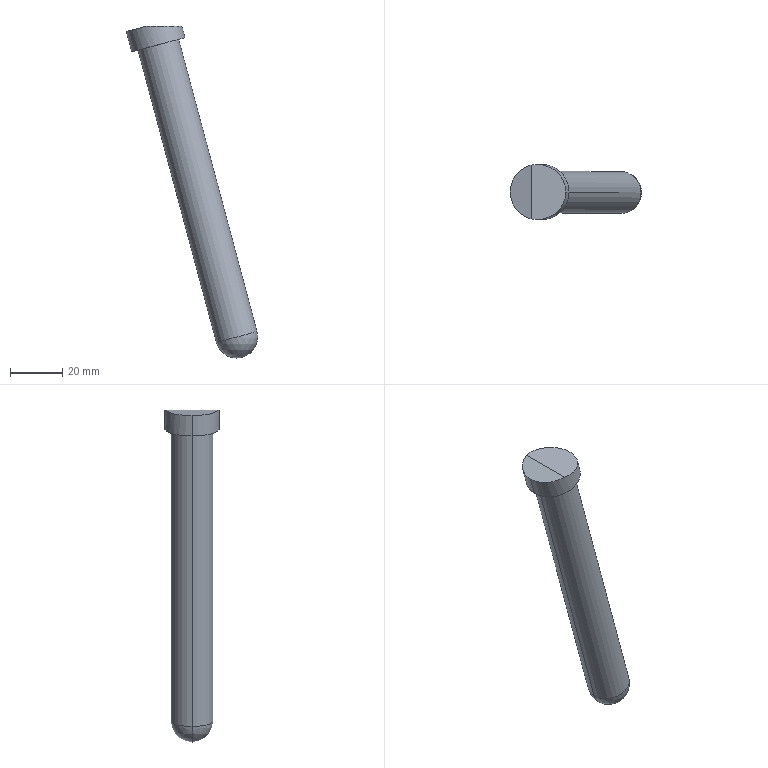Part | Creo | 1 solid | 9 faces | box 50.078 x 21.003 x 126.591 mm | volume 26716 mm3 | cylinder 4 | plane 3 | sphere 2 | commonest cylinder face diameters 16 x2 21 x2
STEP:
#1=CARTESIAN_POINT('',(0.,0.,0.));
#2=DIRECTION('',(0.,0.,1.));
#3=DIRECTION('',(1.,0.,0.));
#4=AXIS2_PLACEMENT_3D('',#1,#2,#3);
#5=CARTESIAN_POINT('',(101.425,-60.4,116.084));
#6=VERTEX_POINT('',#5);
#7=CARTESIAN_POINT('',(81.14,-60.4,110.649));
#8=VERTEX_POINT('',#7);
#9=CARTESIAN_POINT('',(91.283,-60.4,113.367));
#10=DIRECTION('',(0.2588,0.,-0.9659));
#11=DIRECTION('',(0.9659,0.,0.2588));
#12=AXIS2_PLACEMENT_3D('',#9,#10,#11);
#13=CIRCLE('',#12,10.5);
#14=EDGE_CURVE('',#6,#8,#13,.T.);
#15=ORIENTED_EDGE('',*,*,#14,.T.);
#16=CARTESIAN_POINT('',(79.07,-60.4,118.376));
#17=VERTEX_POINT('',#16);
#18=CARTESIAN_POINT('',(81.14,-60.4,110.649));
#19=DIRECTION('',(-0.2588,0.,0.9659));
#20=VECTOR('',#19,8.);
#21=LINE('',#18,#20);
#22=EDGE_CURVE('',#8,#17,#21,.T.);
#23=ORIENTED_EDGE('',*,*,#22,.T.);
#24=CARTESIAN_POINT('',(86.995,-70.646,120.5));
#25=VERTEX_POINT('',#24);
#26=CARTESIAN_POINT('',(89.212,-60.4,121.094));
#27=DIRECTION('',(-0.2588,0.,0.9659));
#28=DIRECTION('',(-0.9659,0.,-0.2588));
#29=AXIS2_PLACEMENT_3D('',#26,#27,#28);
#30=CIRCLE('',#29,10.5);
#31=EDGE_CURVE('',#17,#25,#30,.T.);
#32=ORIENTED_EDGE('',*,*,#31,.T.);
#33=CARTESIAN_POINT('',(100.242,-60.4,120.5));
#34=VERTEX_POINT('',#33);
#35=CARTESIAN_POINT('',(100.242,-60.4,120.5));
#36=CARTESIAN_POINT('',(100.242,-61.511,120.5));
#37=CARTESIAN_POINT('',(99.914,-63.327,120.5));
#38=CARTESIAN_POINT('',(98.655,-66.211,120.5));
#39=CARTESIAN_POINT('',(96.283,-68.826,120.5));
#40=CARTESIAN_POINT('',(93.114,-70.452,120.5));
#41=CARTESIAN_POINT('',(89.953,-70.979,120.5));
#42=CARTESIAN_POINT('',(88.081,-70.881,120.5));
#43=CARTESIAN_POINT('',(86.995,-70.646,120.5));
#44=B_SPLINE_CURVE_WITH_KNOTS('',3,(#35,#36,#37,#38,#39,#40,#41,#42,#43),.UNSPECIFIED.,.F.,.F.,(4,1,1,1,1,1,4),(0.,0.125,0.25,0.5,0.75,0.875,1.),.UNSPECIFIED.);
#45=EDGE_CURVE('',#34,#25,#44,.T.);
#46=ORIENTED_EDGE('',*,*,#45,.F.);
#47=CARTESIAN_POINT('',(101.425,-60.4,116.084));
#48=DIRECTION('',(-0.2588,0.,0.9659));
#49=VECTOR('',#48,4.572);
#50=LINE('',#47,#49);
#51=EDGE_CURVE('',#6,#34,#50,.T.);
#52=ORIENTED_EDGE('',*,*,#51,.F.);
#53=EDGE_LOOP('',(#15,#23,#32,#46,#52));
#54=FACE_OUTER_BOUND('',#53,.F.);
#55=CARTESIAN_POINT('',(91.283,-60.4,113.367));
#56=DIRECTION('',(-0.2588,0.,0.9659));
#57=DIRECTION('',(-0.9659,0.,-0.2588));
#58=AXIS2_PLACEMENT_3D('',#55,#56,#57);
#59=CYLINDRICAL_SURFACE('',#58,10.5);
#60=ADVANCED_FACE('',(#54),#59,.T.);
#61=CARTESIAN_POINT('',(91.283,-60.4,113.367));
#62=DIRECTION('',(0.2588,0.,-0.9659));
#63=DIRECTION('',(-0.9659,0.,-0.2588));
#64=AXIS2_PLACEMENT_3D('',#61,#62,#63);
#65=CIRCLE('',#64,10.5);
#66=EDGE_CURVE('',#8,#6,#65,.T.);
#67=ORIENTED_EDGE('',*,*,#66,.F.);
#68=ORIENTED_EDGE('',*,*,#14,.F.);
#69=EDGE_LOOP('',(#67,#68));
#70=FACE_OUTER_BOUND('',#69,.F.);
#71=CARTESIAN_POINT('',(83.555,-60.4,111.296));
#72=VERTEX_POINT('',#71);
#73=CARTESIAN_POINT('',(99.01,-60.4,115.437));
#74=VERTEX_POINT('',#73);
#75=CARTESIAN_POINT('',(91.283,-60.4,113.367));
#76=DIRECTION('',(-0.2588,0.,0.9659));
#77=DIRECTION('',(-0.9659,0.,-0.2588));
#78=AXIS2_PLACEMENT_3D('',#75,#76,#77);
#79=CIRCLE('',#78,8.);
#80=EDGE_CURVE('',#72,#74,#79,.T.);
#81=ORIENTED_EDGE('',*,*,#80,.F.);
#82=CARTESIAN_POINT('',(91.283,-60.4,113.367));
#83=DIRECTION('',(-0.2588,0.,0.9659));
#84=DIRECTION('',(0.9659,0.,0.2588));
#85=AXIS2_PLACEMENT_3D('',#82,#83,#84);
#86=CIRCLE('',#85,8.);
#87=EDGE_CURVE('',#74,#72,#86,.T.);
#88=ORIENTED_EDGE('',*,*,#87,.F.);
#89=EDGE_LOOP('',(#81,#88));
#90=FACE_BOUND('',#89,.F.);
#91=CARTESIAN_POINT('',(91.283,-60.4,113.367));
#92=DIRECTION('',(-0.2588,0.,0.9659));
#93=DIRECTION('',(-0.9659,0.,-0.2588));
#94=AXIS2_PLACEMENT_3D('',#91,#92,#93);
#95=PLANE('',#94);
#96=ADVANCED_FACE('',(#70,#90),#95,.F.);
#97=ORIENTED_EDGE('',*,*,#66,.T.);
#98=ORIENTED_EDGE('',*,*,#51,.T.);
#99=CARTESIAN_POINT('',(86.995,-50.154,120.5));
#100=VERTEX_POINT('',#99);
#101=CARTESIAN_POINT('',(100.242,-60.4,120.5));
#102=CARTESIAN_POINT('',(100.242,-59.289,120.5));
#103=CARTESIAN_POINT('',(99.914,-57.473,120.5));
#104=CARTESIAN_POINT('',(98.655,-54.589,120.5));
#105=CARTESIAN_POINT('',(96.283,-51.974,120.5));
#106=CARTESIAN_POINT('',(93.114,-50.348,120.5));
#107=CARTESIAN_POINT('',(89.953,-49.821,120.5));
#108=CARTESIAN_POINT('',(88.081,-49.919,120.5));
#109=CARTESIAN_POINT('',(86.995,-50.154,120.5));
#110=B_SPLINE_CURVE_WITH_KNOTS('',3,(#101,#102,#103,#104,#105,#106,#107,#108,#109),.UNSPECIFIED.,.F.,.F.,(4,1,1,1,1,1,4),(0.,0.125,0.25,0.5,0.75,0.875,1.),.UNSPECIFIED.);
#111=EDGE_CURVE('',#34,#100,#110,.T.);
#112=ORIENTED_EDGE('',*,*,#111,.T.);
#113=CARTESIAN_POINT('',(89.212,-60.4,121.094));
#114=DIRECTION('',(-0.2588,0.,0.9659));
#115=DIRECTION('',(-0.2111,0.9758,-0.05657));
#116=AXIS2_PLACEMENT_3D('',#113,#114,#115);
#117=CIRCLE('',#116,10.5);
#118=EDGE_CURVE('',#100,#17,#117,.T.);
#119=ORIENTED_EDGE('',*,*,#118,.T.);
#120=ORIENTED_EDGE('',*,*,#22,.F.);
#121=EDGE_LOOP('',(#97,#98,#112,#119,#120));
#122=FACE_OUTER_BOUND('',#121,.F.);
#123=CARTESIAN_POINT('',(91.283,-60.4,113.367));
#124=DIRECTION('',(-0.2588,0.,0.9659));
#125=DIRECTION('',(-0.9659,0.,-0.2588));
#126=AXIS2_PLACEMENT_3D('',#123,#124,#125);
#127=CYLINDRICAL_SURFACE('',#126,10.5);
#128=ADVANCED_FACE('',(#122),#127,.T.);
#129=ORIENTED_EDGE('',*,*,#45,.T.);
#130=CARTESIAN_POINT('',(86.995,-50.154,120.5));
#131=DIRECTION('',(0.,-1.,0.));
#132=VECTOR('',#131,20.492);
#133=LINE('',#130,#132);
#134=EDGE_CURVE('',#100,#25,#133,.T.);
#135=ORIENTED_EDGE('',*,*,#134,.F.);
#136=ORIENTED_EDGE('',*,*,#111,.F.);
#137=EDGE_LOOP('',(#129,#135,#136));
#138=FACE_OUTER_BOUND('',#137,.F.);
#139=CARTESIAN_POINT('',(0.,-0.8,120.5));
#140=DIRECTION('',(0.,0.,1.));
#141=DIRECTION('',(-1.,0.,0.));
#142=AXIS2_PLACEMENT_3D('',#139,#140,#141);
#143=PLANE('',#142);
#144=ADVANCED_FACE('',(#138),#143,.T.);
#145=ORIENTED_EDGE('',*,*,#31,.F.);
#146=ORIENTED_EDGE('',*,*,#118,.F.);
#147=ORIENTED_EDGE('',*,*,#134,.T.);
#148=EDGE_LOOP('',(#145,#146,#147));
#149=FACE_OUTER_BOUND('',#148,.F.);
#150=CARTESIAN_POINT('',(89.212,-60.4,121.094));
#151=DIRECTION('',(-0.2588,0.,0.9659));
#152=DIRECTION('',(-0.9659,0.,-0.2588));
#153=AXIS2_PLACEMENT_3D('',#150,#151,#152);
#154=PLANE('',#153);
#155=ADVANCED_FACE('',(#149),#154,.T.);
#156=ORIENTED_EDGE('',*,*,#80,.T.);
#157=CARTESIAN_POINT('',(128.875,-60.4,3.98));
#158=VERTEX_POINT('',#157);
#159=CARTESIAN_POINT('',(128.875,-60.4,3.98));
#160=DIRECTION('',(-0.2588,0.,0.9659));
#161=VECTOR('',#160,115.389);
#162=LINE('',#159,#161);
#163=EDGE_CURVE('',#158,#74,#162,.T.);
#164=ORIENTED_EDGE('',*,*,#163,.F.);
#165=CARTESIAN_POINT('',(113.42,-60.4,-0.1613));
#166=VERTEX_POINT('',#165);
#167=CARTESIAN_POINT('',(121.147,-60.4,1.909));
#168=DIRECTION('',(0.2588,0.,-0.9659));
#169=DIRECTION('',(0.9659,0.,0.2588));
#170=AXIS2_PLACEMENT_3D('',#167,#168,#169);
#171=CIRCLE('',#170,8.);
#172=EDGE_CURVE('',#158,#166,#171,.T.);
#173=ORIENTED_EDGE('',*,*,#172,.T.);
#174=CARTESIAN_POINT('',(113.42,-60.4,-0.1613));
#175=DIRECTION('',(-0.2588,0.,0.9659));
#176=VECTOR('',#175,115.389);
#177=LINE('',#174,#176);
#178=EDGE_CURVE('',#166,#72,#177,.T.);
#179=ORIENTED_EDGE('',*,*,#178,.T.);
#180=EDGE_LOOP('',(#156,#164,#173,#179));
#181=FACE_OUTER_BOUND('',#180,.F.);
#182=CARTESIAN_POINT('',(131.917,-60.4,-38.284));
#183=DIRECTION('',(-0.2588,0.,0.9659));
#184=DIRECTION('',(-0.9659,0.,-0.2588));
#185=AXIS2_PLACEMENT_3D('',#182,#183,#184);
#186=CYLINDRICAL_SURFACE('',#185,8.);
#187=ADVANCED_FACE('',(#181),#186,.T.);
#188=ORIENTED_EDGE('',*,*,#87,.T.);
#189=ORIENTED_EDGE('',*,*,#178,.F.);
#190=CARTESIAN_POINT('',(121.147,-60.4,1.909));
#191=DIRECTION('',(0.2588,0.,-0.9659));
#192=DIRECTION('',(-0.9659,0.,-0.2588));
#193=AXIS2_PLACEMENT_3D('',#190,#191,#192);
#194=CIRCLE('',#193,8.);
#195=EDGE_CURVE('',#166,#158,#194,.T.);
#196=ORIENTED_EDGE('',*,*,#195,.T.);
#197=ORIENTED_EDGE('',*,*,#163,.T.);
#198=EDGE_LOOP('',(#188,#189,#196,#197));
#199=FACE_OUTER_BOUND('',#198,.F.);
#200=CARTESIAN_POINT('',(131.917,-60.4,-38.284));
#201=DIRECTION('',(-0.2588,0.,0.9659));
#202=DIRECTION('',(-0.9659,0.,-0.2588));
#203=AXIS2_PLACEMENT_3D('',#200,#201,#202);
#204=CYLINDRICAL_SURFACE('',#203,8.);
#205=ADVANCED_FACE('',(#199),#204,.T.);
#206=ORIENTED_EDGE('',*,*,#195,.F.);
#207=CARTESIAN_POINT('',(121.147,-60.4,-6.091));
#208=VERTEX_POINT('',#207);
#209=CARTESIAN_POINT('',(121.147,-60.4,1.909));
#210=DIRECTION('',(0.,1.,0.));
#211=DIRECTION('',(0.,0.,-1.));
#212=AXIS2_PLACEMENT_3D('',#209,#210,#211);
#213=CIRCLE('',#212,8.);
#214=EDGE_CURVE('',#208,#166,#213,.T.);
#215=ORIENTED_EDGE('',*,*,#214,.F.);
#216=CARTESIAN_POINT('',(121.147,-60.4,1.909));
#217=DIRECTION('',(0.,-1.,0.));
#218=DIRECTION('',(0.,0.,-1.));
#219=AXIS2_PLACEMENT_3D('',#216,#217,#218);
#220=CIRCLE('',#219,8.);
#221=EDGE_CURVE('',#208,#158,#220,.T.);
#222=ORIENTED_EDGE('',*,*,#221,.T.);
#223=EDGE_LOOP('',(#206,#215,#222));
#224=FACE_OUTER_BOUND('',#223,.F.);
#225=CARTESIAN_POINT('',(121.147,-60.4,1.909));
#226=DIRECTION('',(0.,0.,1.));
#227=DIRECTION('',(-1.,0.,0.));
#228=AXIS2_PLACEMENT_3D('',#225,#226,#227);
#229=SPHERICAL_SURFACE('',#228,8.);
#230=ADVANCED_FACE('',(#224),#229,.T.);
#231=ORIENTED_EDGE('',*,*,#172,.F.);
#232=ORIENTED_EDGE('',*,*,#221,.F.);
#233=ORIENTED_EDGE('',*,*,#214,.T.);
#234=EDGE_LOOP('',(#231,#232,#233));
#235=FACE_OUTER_BOUND('',#234,.F.);
#236=CARTESIAN_POINT('',(121.147,-60.4,1.909));
#237=DIRECTION('',(0.,0.,1.));
#238=DIRECTION('',(-1.,0.,0.));
#239=AXIS2_PLACEMENT_3D('',#236,#237,#238);
#240=SPHERICAL_SURFACE('',#239,8.);
#241=ADVANCED_FACE('',(#235),#240,.T.);
#242=CLOSED_SHELL('',(#60,#96,#128,#144,#155,#187,#205,#230,#241));
#243=MANIFOLD_SOLID_BREP('',#242);
#244=(LENGTH_UNIT()NAMED_UNIT(*)SI_UNIT(.MILLI.,.METRE.));
#245=UNCERTAINTY_MEASURE_WITH_UNIT(LENGTH_MEASURE(0.01408),#244,'','');
#246=(NAMED_UNIT(*)PLANE_ANGLE_UNIT()SI_UNIT($,.RADIAN.));
#247=PLANE_ANGLE_MEASURE_WITH_UNIT(PLANE_ANGLE_MEASURE(0.01745),#246);
#248=(CONVERSION_BASED_UNIT('DEGREE',#247)NAMED_UNIT(*)PLANE_ANGLE_UNIT());
#249=(NAMED_UNIT(*)SI_UNIT($,.STERADIAN.)SOLID_ANGLE_UNIT());
#250=(GEOMETRIC_REPRESENTATION_CONTEXT(3)GLOBAL_UNCERTAINTY_ASSIGNED_CONTEXT((#245))GLOBAL_UNIT_ASSIGNED_CONTEXT((#244,#248,#249))REPRESENTATION_CONTEXT('',''));
#251=ADVANCED_BREP_SHAPE_REPRESENTATION('',(#4,#243),#250);